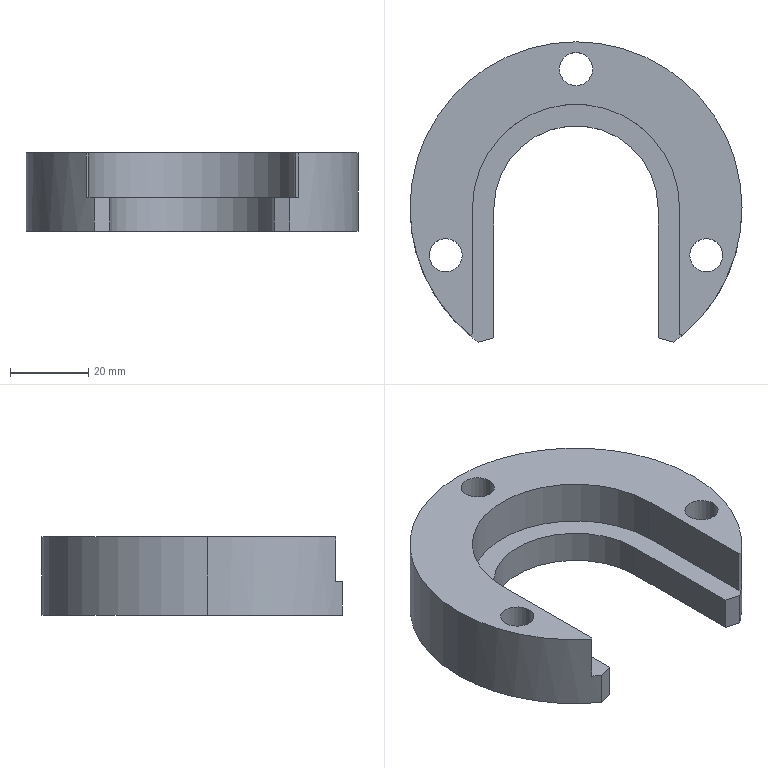Part | STEP file | Cylinder Gland 2 | 1 solid | 22 faces | box 85 x 76.879 x 20 mm | volume 52737 mm3 | cylinder 11 | plane 11 | commonest cylinder face diameters 8.5 x6 85 x3 42 x1 53 x1